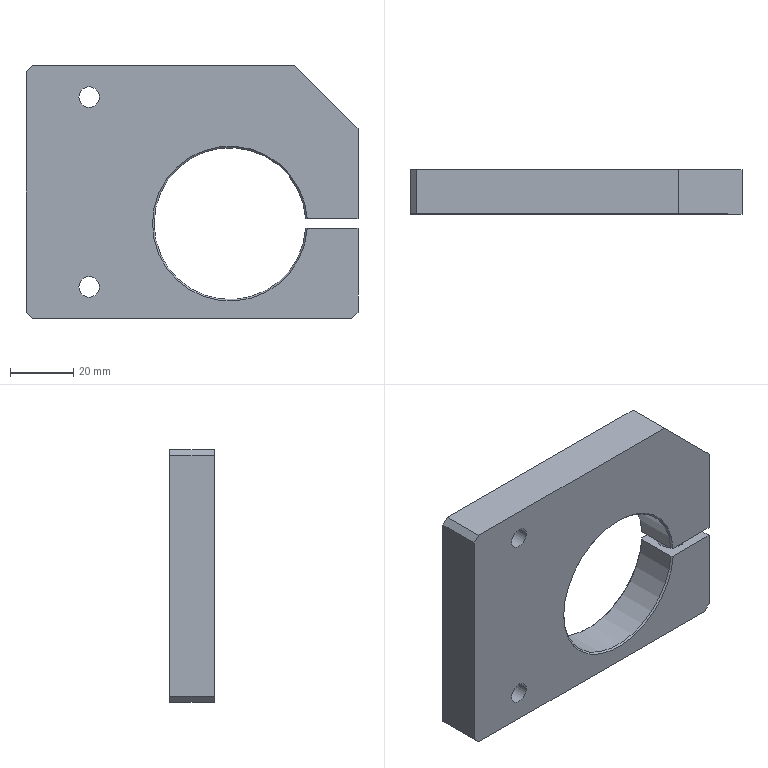Part | NX | 1 solid | 30 faces | box 105 x 14 x 80 mm | volume 85022 mm3 | plane 13 | cylinder 10 | cone 7 | commonest cylinder face diameters 6.5 x4 6.8 x2 9 x2 48 x2
STEP:
#1=CARTESIAN_POINT('',(-50.5,-7.,-40.));
#2=VERTEX_POINT('',#1);
#3=CARTESIAN_POINT('',(-50.5,7.,-40.));
#4=VERTEX_POINT('',#3);
#5=CARTESIAN_POINT('',(-50.5,-7.,-40.));
#6=DIRECTION('',(0.,1.,0.));
#7=VECTOR('',#6,1000.);
#8=LINE('',#5,#7);
#9=EDGE_CURVE('',#2,#4,#8,.T.);
#10=ORIENTED_EDGE('',*,*,#9,.T.);
#11=CARTESIAN_POINT('',(50.5,7.,-40.));
#12=VERTEX_POINT('',#11);
#13=CARTESIAN_POINT('',(-50.5,7.,-40.));
#14=DIRECTION('',(1.,0.,0.));
#15=VECTOR('',#14,1000.);
#16=LINE('',#13,#15);
#17=EDGE_CURVE('',#4,#12,#16,.T.);
#18=ORIENTED_EDGE('',*,*,#17,.T.);
#19=CARTESIAN_POINT('',(50.5,-7.,-40.));
#20=VERTEX_POINT('',#19);
#21=CARTESIAN_POINT('',(50.5,7.,-40.));
#22=DIRECTION('',(0.,-1.,0.));
#23=VECTOR('',#22,1000.);
#24=LINE('',#21,#23);
#25=EDGE_CURVE('',#12,#20,#24,.T.);
#26=ORIENTED_EDGE('',*,*,#25,.T.);
#27=CARTESIAN_POINT('',(50.5,-7.,-40.));
#28=DIRECTION('',(-1.,0.,0.));
#29=VECTOR('',#28,1000.);
#30=LINE('',#27,#29);
#31=EDGE_CURVE('',#20,#2,#30,.T.);
#32=ORIENTED_EDGE('',*,*,#31,.T.);
#33=EDGE_LOOP('',(#10,#18,#26,#32));
#34=FACE_BOUND('',#33,.T.);
#35=CARTESIAN_POINT('',(47.,0.,-40.));
#36=VERTEX_POINT('',#35);
#37=CARTESIAN_POINT('',(38.,0.,-40.));
#38=VERTEX_POINT('',#37);
#39=CARTESIAN_POINT('',(42.5,0.,-40.));
#40=DIRECTION('',(0.,0.,-1.));
#41=DIRECTION('',(1.,0.,0.));
#42=AXIS2_PLACEMENT_3D('',#39,#40,#41);
#43=CIRCLE('',#42,4.5);
#44=EDGE_CURVE('',#36,#38,#43,.T.);
#45=ORIENTED_EDGE('',*,*,#44,.F.);
#46=CARTESIAN_POINT('',(42.5,0.,-40.));
#47=DIRECTION('',(0.,0.,-1.));
#48=DIRECTION('',(1.,0.,0.));
#49=AXIS2_PLACEMENT_3D('',#46,#47,#48);
#50=CIRCLE('',#49,4.5);
#51=EDGE_CURVE('',#38,#36,#50,.T.);
#52=ORIENTED_EDGE('',*,*,#51,.F.);
#53=EDGE_LOOP('',(#45,#52));
#54=FACE_BOUND('',#53,.T.);
#55=CARTESIAN_POINT('',(0.,0.,-40.));
#56=DIRECTION('',(0.,0.,1.));
#57=DIRECTION('',(1.,0.,0.));
#58=AXIS2_PLACEMENT_3D('',#55,#56,#57);
#59=PLANE('',#58);
#60=ADVANCED_FACE('',(#34,#54),#59,.F.);
#61=ORIENTED_EDGE('',*,*,#9,.F.);
#62=CARTESIAN_POINT('',(-52.5,-7.,-38.));
#63=VERTEX_POINT('',#62);
#64=CARTESIAN_POINT('',(-50.5,-7.,-40.));
#65=DIRECTION('',(-0.7071,0.,0.7071));
#66=VECTOR('',#65,1000.);
#67=LINE('',#64,#66);
#68=EDGE_CURVE('',#2,#63,#67,.T.);
#69=ORIENTED_EDGE('',*,*,#68,.T.);
#70=CARTESIAN_POINT('',(-52.5,7.,-38.));
#71=VERTEX_POINT('',#70);
#72=CARTESIAN_POINT('',(-52.5,-7.,-38.));
#73=DIRECTION('',(0.,1.,0.));
#74=VECTOR('',#73,1000.);
#75=LINE('',#72,#74);
#76=EDGE_CURVE('',#63,#71,#75,.T.);
#77=ORIENTED_EDGE('',*,*,#76,.T.);
#78=CARTESIAN_POINT('',(-52.5,7.,-38.));
#79=DIRECTION('',(0.7071,0.,-0.7071));
#80=VECTOR('',#79,1000.);
#81=LINE('',#78,#80);
#82=EDGE_CURVE('',#71,#4,#81,.T.);
#83=ORIENTED_EDGE('',*,*,#82,.T.);
#84=EDGE_LOOP('',(#61,#69,#77,#83));
#85=FACE_BOUND('',#84,.T.);
#86=CARTESIAN_POINT('',(-50.5,7.,-40.));
#87=DIRECTION('',(-0.7071,0.,-0.7071));
#88=DIRECTION('',(-0.7071,0.,0.7071));
#89=AXIS2_PLACEMENT_3D('',#86,#87,#88);
#90=PLANE('',#89);
#91=ADVANCED_FACE('',(#85),#90,.T.);
#92=CARTESIAN_POINT('',(36.454,7.,-11.5));
#93=VERTEX_POINT('',#92);
#94=CARTESIAN_POINT('',(52.5,7.,-11.5));
#95=VERTEX_POINT('',#94);
#96=CARTESIAN_POINT('',(36.454,7.,-11.5));
#97=DIRECTION('',(1.,0.,0.));
#98=VECTOR('',#97,1000.);
#99=LINE('',#96,#98);
#100=EDGE_CURVE('',#93,#95,#99,.T.);
#101=ORIENTED_EDGE('',*,*,#100,.T.);
#102=CARTESIAN_POINT('',(52.5,7.,-38.));
#103=VERTEX_POINT('',#102);
#104=CARTESIAN_POINT('',(52.5,7.,-11.5));
#105=DIRECTION('',(0.,0.,-1.));
#106=VECTOR('',#105,1000.);
#107=LINE('',#104,#106);
#108=EDGE_CURVE('',#95,#103,#107,.T.);
#109=ORIENTED_EDGE('',*,*,#108,.T.);
#110=CARTESIAN_POINT('',(50.5,7.,-40.));
#111=DIRECTION('',(0.7071,0.,0.7071));
#112=VECTOR('',#111,1000.);
#113=LINE('',#110,#112);
#114=EDGE_CURVE('',#12,#103,#113,.T.);
#115=ORIENTED_EDGE('',*,*,#114,.F.);
#116=ORIENTED_EDGE('',*,*,#17,.F.);
#117=ORIENTED_EDGE('',*,*,#82,.F.);
#118=CARTESIAN_POINT('',(-52.5,7.,38.));
#119=VERTEX_POINT('',#118);
#120=CARTESIAN_POINT('',(-52.5,7.,38.));
#121=DIRECTION('',(0.,0.,-1.));
#122=VECTOR('',#121,1000.);
#123=LINE('',#120,#122);
#124=EDGE_CURVE('',#119,#71,#123,.T.);
#125=ORIENTED_EDGE('',*,*,#124,.F.);
#126=CARTESIAN_POINT('',(-50.5,7.,40.));
#127=VERTEX_POINT('',#126);
#128=CARTESIAN_POINT('',(-50.5,7.,40.));
#129=DIRECTION('',(-0.7071,0.,-0.7071));
#130=VECTOR('',#129,1000.);
#131=LINE('',#128,#130);
#132=EDGE_CURVE('',#127,#119,#131,.T.);
#133=ORIENTED_EDGE('',*,*,#132,.F.);
#134=CARTESIAN_POINT('',(32.5,7.,40.));
#135=VERTEX_POINT('',#134);
#136=CARTESIAN_POINT('',(-50.5,7.,40.));
#137=DIRECTION('',(1.,0.,0.));
#138=VECTOR('',#137,1000.);
#139=LINE('',#136,#138);
#140=EDGE_CURVE('',#127,#135,#139,.T.);
#141=ORIENTED_EDGE('',*,*,#140,.T.);
#142=CARTESIAN_POINT('',(52.5,7.,20.));
#143=VERTEX_POINT('',#142);
#144=CARTESIAN_POINT('',(52.5,7.,20.));
#145=DIRECTION('',(-0.7071,0.,0.7071));
#146=VECTOR('',#145,1000.);
#147=LINE('',#144,#146);
#148=EDGE_CURVE('',#143,#135,#147,.T.);
#149=ORIENTED_EDGE('',*,*,#148,.F.);
#150=CARTESIAN_POINT('',(52.5,7.,-8.5));
#151=VERTEX_POINT('',#150);
#152=CARTESIAN_POINT('',(52.5,7.,20.));
#153=DIRECTION('',(0.,0.,-1.));
#154=VECTOR('',#153,1000.);
#155=LINE('',#152,#154);
#156=EDGE_CURVE('',#143,#151,#155,.T.);
#157=ORIENTED_EDGE('',*,*,#156,.T.);
#158=CARTESIAN_POINT('',(36.454,7.,-8.5));
#159=VERTEX_POINT('',#158);
#160=CARTESIAN_POINT('',(0.,7.,-8.5));
#161=DIRECTION('',(1.,0.,0.));
#162=VECTOR('',#161,1000.);
#163=LINE('',#160,#162);
#164=EDGE_CURVE('',#159,#151,#163,.T.);
#165=ORIENTED_EDGE('',*,*,#164,.F.);
#166=CARTESIAN_POINT('',(12.,7.,-10.));
#167=DIRECTION('',(0.,1.,0.));
#168=DIRECTION('',(-1.,0.,0.));
#169=AXIS2_PLACEMENT_3D('',#166,#167,#168);
#170=CIRCLE('',#169,24.5);
#171=EDGE_CURVE('',#93,#159,#170,.T.);
#172=ORIENTED_EDGE('',*,*,#171,.F.);
#173=EDGE_LOOP('',(#101,#109,#115,#116,#117,#125,#133,#141,#149,#157,#165,#172));
#174=FACE_BOUND('',#173,.T.);
#175=CARTESIAN_POINT('',(-35.75,7.,30.));
#176=VERTEX_POINT('',#175);
#177=CARTESIAN_POINT('',(-29.25,7.,30.));
#178=VERTEX_POINT('',#177);
#179=CARTESIAN_POINT('',(-32.5,7.,30.));
#180=DIRECTION('',(0.,1.,0.));
#181=DIRECTION('',(1.,0.,0.));
#182=AXIS2_PLACEMENT_3D('',#179,#180,#181);
#183=CIRCLE('',#182,3.25);
#184=EDGE_CURVE('',#176,#178,#183,.T.);
#185=ORIENTED_EDGE('',*,*,#184,.F.);
#186=CARTESIAN_POINT('',(-32.5,7.,30.));
#187=DIRECTION('',(0.,1.,0.));
#188=DIRECTION('',(1.,0.,0.));
#189=AXIS2_PLACEMENT_3D('',#186,#187,#188);
#190=CIRCLE('',#189,3.25);
#191=EDGE_CURVE('',#178,#176,#190,.T.);
#192=ORIENTED_EDGE('',*,*,#191,.F.);
#193=EDGE_LOOP('',(#185,#192));
#194=FACE_BOUND('',#193,.T.);
#195=CARTESIAN_POINT('',(-29.25,7.,-30.));
#196=VERTEX_POINT('',#195);
#197=CARTESIAN_POINT('',(-35.75,7.,-30.));
#198=VERTEX_POINT('',#197);
#199=CARTESIAN_POINT('',(-32.5,7.,-30.));
#200=DIRECTION('',(0.,1.,0.));
#201=DIRECTION('',(1.,0.,0.));
#202=AXIS2_PLACEMENT_3D('',#199,#200,#201);
#203=CIRCLE('',#202,3.25);
#204=EDGE_CURVE('',#196,#198,#203,.T.);
#205=ORIENTED_EDGE('',*,*,#204,.F.);
#206=CARTESIAN_POINT('',(-32.5,7.,-30.));
#207=DIRECTION('',(0.,1.,0.));
#208=DIRECTION('',(1.,0.,0.));
#209=AXIS2_PLACEMENT_3D('',#206,#207,#208);
#210=CIRCLE('',#209,3.25);
#211=EDGE_CURVE('',#198,#196,#210,.T.);
#212=ORIENTED_EDGE('',*,*,#211,.F.);
#213=EDGE_LOOP('',(#205,#212));
#214=FACE_BOUND('',#213,.T.);
#215=CARTESIAN_POINT('',(52.5,7.,-40.));
#216=DIRECTION('',(0.,1.,0.));
#217=DIRECTION('',(1.,0.,0.));
#218=AXIS2_PLACEMENT_3D('',#215,#216,#217);
#219=PLANE('',#218);
#220=ADVANCED_FACE('',(#174,#194,#214),#219,.T.);
#221=CARTESIAN_POINT('',(36.454,-7.,-11.5));
#222=VERTEX_POINT('',#221);
#223=CARTESIAN_POINT('',(52.5,-7.,-11.5));
#224=VERTEX_POINT('',#223);
#225=CARTESIAN_POINT('',(36.454,-7.,-11.5));
#226=DIRECTION('',(1.,0.,0.));
#227=VECTOR('',#226,1000.);
#228=LINE('',#225,#227);
#229=EDGE_CURVE('',#222,#224,#228,.T.);
#230=ORIENTED_EDGE('',*,*,#229,.T.);
#231=CARTESIAN_POINT('',(52.5,7.,-11.5));
#232=DIRECTION('',(0.,-1.,0.));
#233=VECTOR('',#232,1000.);
#234=LINE('',#231,#233);
#235=EDGE_CURVE('',#95,#224,#234,.T.);
#236=ORIENTED_EDGE('',*,*,#235,.F.);
#237=ORIENTED_EDGE('',*,*,#100,.F.);
#238=CARTESIAN_POINT('',(35.953,6.5,-11.5));
#239=VERTEX_POINT('',#238);
#240=CARTESIAN_POINT('',(36.454,7.,-11.5));
#241=CARTESIAN_POINT('',(36.398,6.944,-11.5));
#242=CARTESIAN_POINT('',(36.287,6.833,-11.5));
#243=CARTESIAN_POINT('',(36.12,6.667,-11.5));
#244=CARTESIAN_POINT('',(36.009,6.556,-11.5));
#245=CARTESIAN_POINT('',(35.953,6.5,-11.5));
#246=B_SPLINE_CURVE_WITH_KNOTS('',3,(#240,#241,#242,#243,#244,#245),.UNSPECIFIED.,.F.,.F.,(4,1,1,4),(0.,0.3333,0.6667,1.),.UNSPECIFIED.);
#247=EDGE_CURVE('',#93,#239,#246,.T.);
#248=ORIENTED_EDGE('',*,*,#247,.T.);
#249=CARTESIAN_POINT('',(35.953,-6.5,-11.5));
#250=VERTEX_POINT('',#249);
#251=CARTESIAN_POINT('',(35.953,6.5,-11.5));
#252=DIRECTION('',(0.,-1.,0.));
#253=VECTOR('',#252,1000.);
#254=LINE('',#251,#253);
#255=EDGE_CURVE('',#239,#250,#254,.T.);
#256=ORIENTED_EDGE('',*,*,#255,.T.);
#257=CARTESIAN_POINT('',(35.953,-6.5,-11.5));
#258=CARTESIAN_POINT('',(36.009,-6.556,-11.5));
#259=CARTESIAN_POINT('',(36.12,-6.667,-11.5));
#260=CARTESIAN_POINT('',(36.287,-6.833,-11.5));
#261=CARTESIAN_POINT('',(36.398,-6.944,-11.5));
#262=CARTESIAN_POINT('',(36.454,-7.,-11.5));
#263=B_SPLINE_CURVE_WITH_KNOTS('',3,(#257,#258,#259,#260,#261,#262),.UNSPECIFIED.,.F.,.F.,(4,1,1,4),(0.,0.3333,0.6667,1.),.UNSPECIFIED.);
#264=EDGE_CURVE('',#250,#222,#263,.T.);
#265=ORIENTED_EDGE('',*,*,#264,.T.);
#266=EDGE_LOOP('',(#230,#236,#237,#248,#256,#265));
#267=FACE_BOUND('',#266,.T.);
#268=CARTESIAN_POINT('',(47.,0.,-11.5));
#269=VERTEX_POINT('',#268);
#270=CARTESIAN_POINT('',(38.,0.,-11.5));
#271=VERTEX_POINT('',#270);
#272=CARTESIAN_POINT('',(42.5,0.,-11.5));
#273=DIRECTION('',(0.,0.,1.));
#274=DIRECTION('',(-1.,0.,0.));
#275=AXIS2_PLACEMENT_3D('',#272,#273,#274);
#276=CIRCLE('',#275,4.5);
#277=EDGE_CURVE('',#269,#271,#276,.T.);
#278=ORIENTED_EDGE('',*,*,#277,.F.);
#279=CARTESIAN_POINT('',(42.5,0.,-11.5));
#280=DIRECTION('',(0.,0.,1.));
#281=DIRECTION('',(-1.,0.,0.));
#282=AXIS2_PLACEMENT_3D('',#279,#280,#281);
#283=CIRCLE('',#282,4.5);
#284=EDGE_CURVE('',#271,#269,#283,.T.);
#285=ORIENTED_EDGE('',*,*,#284,.F.);
#286=EDGE_LOOP('',(#278,#285));
#287=FACE_BOUND('',#286,.T.);
#288=CARTESIAN_POINT('',(52.5,7.,-11.5));
#289=DIRECTION('',(0.,0.,-1.));
#290=DIRECTION('',(0.,-1.,0.));
#291=AXIS2_PLACEMENT_3D('',#288,#289,#290);
#292=PLANE('',#291);
#293=ADVANCED_FACE('',(#267,#287),#292,.F.);
#294=ORIENTED_EDGE('',*,*,#229,.F.);
#295=CARTESIAN_POINT('',(-12.5,-7.,-10.));
#296=VERTEX_POINT('',#295);
#297=CARTESIAN_POINT('',(12.,-7.,-10.));
#298=DIRECTION('',(0.,-1.,0.));
#299=DIRECTION('',(-1.,0.,0.));
#300=AXIS2_PLACEMENT_3D('',#297,#298,#299);
#301=CIRCLE('',#300,24.5);
#302=EDGE_CURVE('',#296,#222,#301,.T.);
#303=ORIENTED_EDGE('',*,*,#302,.F.);
#304=CARTESIAN_POINT('',(36.454,-7.,-8.5));
#305=VERTEX_POINT('',#304);
#306=CARTESIAN_POINT('',(12.,-7.,-10.));
#307=DIRECTION('',(0.,-1.,0.));
#308=DIRECTION('',(-1.,0.,0.));
#309=AXIS2_PLACEMENT_3D('',#306,#307,#308);
#310=CIRCLE('',#309,24.5);
#311=EDGE_CURVE('',#305,#296,#310,.T.);
#312=ORIENTED_EDGE('',*,*,#311,.F.);
#313=CARTESIAN_POINT('',(52.5,-7.,-8.5));
#314=VERTEX_POINT('',#313);
#315=CARTESIAN_POINT('',(0.,-7.,-8.5));
#316=DIRECTION('',(-1.,0.,0.));
#317=VECTOR('',#316,1000.);
#318=LINE('',#315,#317);
#319=EDGE_CURVE('',#314,#305,#318,.T.);
#320=ORIENTED_EDGE('',*,*,#319,.F.);
#321=CARTESIAN_POINT('',(52.5,-7.,20.));
#322=VERTEX_POINT('',#321);
#323=CARTESIAN_POINT('',(52.5,-7.,20.));
#324=DIRECTION('',(0.,0.,-1.));
#325=VECTOR('',#324,1000.);
#326=LINE('',#323,#325);
#327=EDGE_CURVE('',#322,#314,#326,.T.);
#328=ORIENTED_EDGE('',*,*,#327,.F.);
#329=CARTESIAN_POINT('',(32.5,-7.,40.));
#330=VERTEX_POINT('',#329);
#331=CARTESIAN_POINT('',(32.5,-7.,40.));
#332=DIRECTION('',(0.7071,0.,-0.7071));
#333=VECTOR('',#332,1000.);
#334=LINE('',#331,#333);
#335=EDGE_CURVE('',#330,#322,#334,.T.);
#336=ORIENTED_EDGE('',*,*,#335,.F.);
#337=CARTESIAN_POINT('',(-50.5,-7.,40.));
#338=VERTEX_POINT('',#337);
#339=CARTESIAN_POINT('',(32.5,-7.,40.));
#340=DIRECTION('',(-1.,0.,0.));
#341=VECTOR('',#340,1000.);
#342=LINE('',#339,#341);
#343=EDGE_CURVE('',#330,#338,#342,.T.);
#344=ORIENTED_EDGE('',*,*,#343,.T.);
#345=CARTESIAN_POINT('',(-52.5,-7.,38.));
#346=VERTEX_POINT('',#345);
#347=CARTESIAN_POINT('',(-52.5,-7.,38.));
#348=DIRECTION('',(0.7071,0.,0.7071));
#349=VECTOR('',#348,1000.);
#350=LINE('',#347,#349);
#351=EDGE_CURVE('',#346,#338,#350,.T.);
#352=ORIENTED_EDGE('',*,*,#351,.F.);
#353=CARTESIAN_POINT('',(-52.5,-7.,38.));
#354=DIRECTION('',(0.,0.,-1.));
#355=VECTOR('',#354,1000.);
#356=LINE('',#353,#355);
#357=EDGE_CURVE('',#346,#63,#356,.T.);
#358=ORIENTED_EDGE('',*,*,#357,.T.);
#359=ORIENTED_EDGE('',*,*,#68,.F.);
#360=ORIENTED_EDGE('',*,*,#31,.F.);
#361=CARTESIAN_POINT('',(52.5,-7.,-38.));
#362=VERTEX_POINT('',#361);
#363=CARTESIAN_POINT('',(52.5,-7.,-38.));
#364=DIRECTION('',(-0.7071,0.,-0.7071));
#365=VECTOR('',#364,1000.);
#366=LINE('',#363,#365);
#367=EDGE_CURVE('',#362,#20,#366,.T.);
#368=ORIENTED_EDGE('',*,*,#367,.F.);
#369=CARTESIAN_POINT('',(52.5,-7.,-11.5));
#370=DIRECTION('',(0.,0.,-1.));
#371=VECTOR('',#370,1000.);
#372=LINE('',#369,#371);
#373=EDGE_CURVE('',#224,#362,#372,.T.);
#374=ORIENTED_EDGE('',*,*,#373,.F.);
#375=EDGE_LOOP('',(#294,#303,#312,#320,#328,#336,#344,#352,#358,#359,#360,#368,#374));
#376=FACE_BOUND('',#375,.T.);
#377=CARTESIAN_POINT('',(-35.75,-7.,30.));
#378=VERTEX_POINT('',#377);
#379=CARTESIAN_POINT('',(-29.25,-7.,30.));
#380=VERTEX_POINT('',#379);
#381=CARTESIAN_POINT('',(-32.5,-7.,30.));
#382=DIRECTION('',(0.,-1.,0.));
#383=DIRECTION('',(-1.,0.,0.));
#384=AXIS2_PLACEMENT_3D('',#381,#382,#383);
#385=CIRCLE('',#384,3.25);
#386=EDGE_CURVE('',#378,#380,#385,.T.);
#387=ORIENTED_EDGE('',*,*,#386,.F.);
#388=CARTESIAN_POINT('',(-32.5,-7.,30.));
#389=DIRECTION('',(0.,-1.,0.));
#390=DIRECTION('',(-1.,0.,0.));
#391=AXIS2_PLACEMENT_3D('',#388,#389,#390);
#392=CIRCLE('',#391,3.25);
#393=EDGE_CURVE('',#380,#378,#392,.T.);
#394=ORIENTED_EDGE('',*,*,#393,.F.);
#395=EDGE_LOOP('',(#387,#394));
#396=FACE_BOUND('',#395,.T.);
#397=CARTESIAN_POINT('',(-29.25,-7.,-30.));
#398=VERTEX_POINT('',#397);
#399=CARTESIAN_POINT('',(-35.75,-7.,-30.));
#400=VERTEX_POINT('',#399);
#401=CARTESIAN_POINT('',(-32.5,-7.,-30.));
#402=DIRECTION('',(0.,-1.,0.));
#403=DIRECTION('',(-1.,0.,0.));
#404=AXIS2_PLACEMENT_3D('',#401,#402,#403);
#405=CIRCLE('',#404,3.25);
#406=EDGE_CURVE('',#398,#400,#405,.T.);
#407=ORIENTED_EDGE('',*,*,#406,.F.);
#408=CARTESIAN_POINT('',(-32.5,-7.,-30.));
#409=DIRECTION('',(0.,-1.,0.));
#410=DIRECTION('',(-1.,0.,0.));
#411=AXIS2_PLACEMENT_3D('',#408,#409,#410);
#412=CIRCLE('',#411,3.25);
#413=EDGE_CURVE('',#400,#398,#412,.T.);
#414=ORIENTED_EDGE('',*,*,#413,.F.);
#415=EDGE_LOOP('',(#407,#414));
#416=FACE_BOUND('',#415,.T.);
#417=CARTESIAN_POINT('',(-52.5,-7.,-40.));
#418=DIRECTION('',(0.,-1.,0.));
#419=DIRECTION('',(0.,0.,-1.));
#420=AXIS2_PLACEMENT_3D('',#417,#418,#419);
#421=PLANE('',#420);
#422=ADVANCED_FACE('',(#376,#396,#416),#421,.T.);
#423=ORIENTED_EDGE('',*,*,#235,.T.);
#424=ORIENTED_EDGE('',*,*,#373,.T.);
#425=CARTESIAN_POINT('',(52.5,7.,-38.));
#426=DIRECTION('',(0.,-1.,0.));
#427=VECTOR('',#426,1000.);
#428=LINE('',#425,#427);
#429=EDGE_CURVE('',#103,#362,#428,.T.);
#430=ORIENTED_EDGE('',*,*,#429,.F.);
#431=ORIENTED_EDGE('',*,*,#108,.F.);
#432=EDGE_LOOP('',(#423,#424,#430,#431));
#433=FACE_BOUND('',#432,.T.);
#434=CARTESIAN_POINT('',(52.5,-7.,-40.));
#435=DIRECTION('',(1.,0.,0.));
#436=DIRECTION('',(0.,1.,0.));
#437=AXIS2_PLACEMENT_3D('',#434,#435,#436);
#438=PLANE('',#437);
#439=ADVANCED_FACE('',(#433),#438,.T.);
#440=ORIENTED_EDGE('',*,*,#25,.F.);
#441=ORIENTED_EDGE('',*,*,#114,.T.);
#442=ORIENTED_EDGE('',*,*,#429,.T.);
#443=ORIENTED_EDGE('',*,*,#367,.T.);
#444=EDGE_LOOP('',(#440,#441,#442,#443));
#445=FACE_BOUND('',#444,.T.);
#446=CARTESIAN_POINT('',(50.5,-7.,-40.));
#447=DIRECTION('',(0.7071,0.,-0.7071));
#448=DIRECTION('',(0.,-1.,0.));
#449=AXIS2_PLACEMENT_3D('',#446,#447,#448);
#450=PLANE('',#449);
#451=ADVANCED_FACE('',(#445),#450,.T.);
#452=ORIENTED_EDGE('',*,*,#76,.F.);
#453=ORIENTED_EDGE('',*,*,#357,.F.);
#454=CARTESIAN_POINT('',(-52.5,-7.,38.));
#455=DIRECTION('',(0.,1.,0.));
#456=VECTOR('',#455,1000.);
#457=LINE('',#454,#456);
#458=EDGE_CURVE('',#346,#119,#457,.T.);
#459=ORIENTED_EDGE('',*,*,#458,.T.);
#460=ORIENTED_EDGE('',*,*,#124,.T.);
#461=EDGE_LOOP('',(#452,#453,#459,#460));
#462=FACE_BOUND('',#461,.T.);
#463=CARTESIAN_POINT('',(-52.5,7.,-40.));
#464=DIRECTION('',(-1.,0.,0.));
#465=DIRECTION('',(0.,0.,1.));
#466=AXIS2_PLACEMENT_3D('',#463,#464,#465);
#467=PLANE('',#466);
#468=ADVANCED_FACE('',(#462),#467,.T.);
#469=CARTESIAN_POINT('',(-50.5,-7.,40.));
#470=DIRECTION('',(0.,1.,0.));
#471=VECTOR('',#470,1000.);
#472=LINE('',#469,#471);
#473=EDGE_CURVE('',#338,#127,#472,.T.);
#474=ORIENTED_EDGE('',*,*,#473,.T.);
#475=ORIENTED_EDGE('',*,*,#132,.T.);
#476=ORIENTED_EDGE('',*,*,#458,.F.);
#477=ORIENTED_EDGE('',*,*,#351,.T.);
#478=EDGE_LOOP('',(#474,#475,#476,#477));
#479=FACE_BOUND('',#478,.T.);
#480=CARTESIAN_POINT('',(-50.5,7.,40.));
#481=DIRECTION('',(0.7071,0.,-0.7071));
#482=DIRECTION('',(0.,-1.,0.));
#483=AXIS2_PLACEMENT_3D('',#480,#481,#482);
#484=PLANE('',#483);
#485=ADVANCED_FACE('',(#479),#484,.F.);
#486=ORIENTED_EDGE('',*,*,#473,.F.);
#487=ORIENTED_EDGE('',*,*,#343,.F.);
#488=CARTESIAN_POINT('',(32.5,7.,40.));
#489=DIRECTION('',(0.,-1.,0.));
#490=VECTOR('',#489,1000.);
#491=LINE('',#488,#490);
#492=EDGE_CURVE('',#135,#330,#491,.T.);
#493=ORIENTED_EDGE('',*,*,#492,.F.);
#494=ORIENTED_EDGE('',*,*,#140,.F.);
#495=EDGE_LOOP('',(#486,#487,#493,#494));
#496=FACE_BOUND('',#495,.T.);
#497=CARTESIAN_POINT('',(0.,0.,40.));
#498=DIRECTION('',(0.,0.,1.));
#499=DIRECTION('',(1.,0.,0.));
#500=AXIS2_PLACEMENT_3D('',#497,#498,#499);
#501=PLANE('',#500);
#502=ADVANCED_FACE('',(#496),#501,.T.);
#503=ORIENTED_EDGE('',*,*,#492,.T.);
#504=ORIENTED_EDGE('',*,*,#335,.T.);
#505=CARTESIAN_POINT('',(52.5,7.,20.));
#506=DIRECTION('',(0.,-1.,0.));
#507=VECTOR('',#506,1000.);
#508=LINE('',#505,#507);
#509=EDGE_CURVE('',#143,#322,#508,.T.);
#510=ORIENTED_EDGE('',*,*,#509,.F.);
#511=ORIENTED_EDGE('',*,*,#148,.T.);
#512=EDGE_LOOP('',(#503,#504,#510,#511));
#513=FACE_BOUND('',#512,.T.);
#514=CARTESIAN_POINT('',(32.5,-7.,40.));
#515=DIRECTION('',(-0.7071,0.,-0.7071));
#516=DIRECTION('',(-0.7071,0.,0.7071));
#517=AXIS2_PLACEMENT_3D('',#514,#515,#516);
#518=PLANE('',#517);
#519=ADVANCED_FACE('',(#513),#518,.F.);
#520=CARTESIAN_POINT('',(52.5,0.,-8.5));
#521=DIRECTION('',(0.,-1.,0.));
#522=VECTOR('',#521,1000.);
#523=LINE('',#520,#522);
#524=EDGE_CURVE('',#151,#314,#523,.T.);
#525=ORIENTED_EDGE('',*,*,#524,.F.);
#526=ORIENTED_EDGE('',*,*,#156,.F.);
#527=ORIENTED_EDGE('',*,*,#509,.T.);
#528=ORIENTED_EDGE('',*,*,#327,.T.);
#529=EDGE_LOOP('',(#525,#526,#527,#528));
#530=FACE_BOUND('',#529,.T.);
#531=CARTESIAN_POINT('',(52.5,-7.,-40.));
#532=DIRECTION('',(1.,0.,0.));
#533=DIRECTION('',(0.,1.,0.));
#534=AXIS2_PLACEMENT_3D('',#531,#532,#533);
#535=PLANE('',#534);
#536=ADVANCED_FACE('',(#530),#535,.T.);
#537=ORIENTED_EDGE('',*,*,#319,.T.);
#538=CARTESIAN_POINT('',(35.953,-6.5,-8.5));
#539=VERTEX_POINT('',#538);
#540=CARTESIAN_POINT('',(35.953,-6.5,-8.5));
#541=CARTESIAN_POINT('',(35.995,-6.542,-8.5));
#542=CARTESIAN_POINT('',(36.037,-6.583,-8.5));
#543=CARTESIAN_POINT('',(36.078,-6.625,-8.5));
#544=CARTESIAN_POINT('',(36.12,-6.667,-8.5));
#545=CARTESIAN_POINT('',(36.162,-6.708,-8.5));
#546=CARTESIAN_POINT('',(36.204,-6.75,-8.5));
#547=CARTESIAN_POINT('',(36.245,-6.792,-8.5));
#548=CARTESIAN_POINT('',(36.287,-6.833,-8.5));
#549=CARTESIAN_POINT('',(36.329,-6.875,-8.5));
#550=CARTESIAN_POINT('',(36.371,-6.917,-8.5));
#551=CARTESIAN_POINT('',(36.412,-6.958,-8.5));
#552=CARTESIAN_POINT('',(36.454,-7.,-8.5));
#553=B_SPLINE_CURVE_WITH_KNOTS('',3,(#540,#541,#542,#543,#544,#545,#546,#547,#548,#549,#550,#551,#552),.UNSPECIFIED.,.F.,.F.,(4,3,3,3,4),(0.,0.1769,0.3539,0.5308,0.7078),.UNSPECIFIED.);
#554=EDGE_CURVE('',#539,#305,#553,.T.);
#555=ORIENTED_EDGE('',*,*,#554,.F.);
#556=CARTESIAN_POINT('',(35.953,6.5,-8.5));
#557=VERTEX_POINT('',#556);
#558=CARTESIAN_POINT('',(35.953,-7.,-8.5));
#559=DIRECTION('',(0.,1.,0.));
#560=VECTOR('',#559,1000.);
#561=LINE('',#558,#560);
#562=EDGE_CURVE('',#539,#557,#561,.T.);
#563=ORIENTED_EDGE('',*,*,#562,.T.);
#564=CARTESIAN_POINT('',(36.454,7.,-8.5));
#565=CARTESIAN_POINT('',(36.412,6.958,-8.5));
#566=CARTESIAN_POINT('',(36.371,6.917,-8.5));
#567=CARTESIAN_POINT('',(36.329,6.875,-8.5));
#568=CARTESIAN_POINT('',(36.287,6.833,-8.5));
#569=CARTESIAN_POINT('',(36.245,6.792,-8.5));
#570=CARTESIAN_POINT('',(36.204,6.75,-8.5));
#571=CARTESIAN_POINT('',(36.162,6.708,-8.5));
#572=CARTESIAN_POINT('',(36.12,6.667,-8.5));
#573=CARTESIAN_POINT('',(36.078,6.625,-8.5));
#574=CARTESIAN_POINT('',(36.057,6.604,-8.5));
#575=CARTESIAN_POINT('',(36.037,6.583,-8.5));
#576=CARTESIAN_POINT('',(36.016,6.562,-8.5));
#577=CARTESIAN_POINT('',(35.995,6.542,-8.5));
#578=CARTESIAN_POINT('',(35.974,6.521,-8.5));
#579=CARTESIAN_POINT('',(35.953,6.5,-8.5));
#580=B_SPLINE_CURVE_WITH_KNOTS('',3,(#564,#565,#566,#567,#568,#569,#570,#571,#572,#573,#574,#575,#576,#577,#578,#579),.UNSPECIFIED.,.F.,.F.,(4,3,3,3,3,4),(0.,0.1769,0.3539,0.5308,0.6193,0.7078),.UNSPECIFIED.);
#581=EDGE_CURVE('',#159,#557,#580,.T.);
#582=ORIENTED_EDGE('',*,*,#581,.F.);
#583=ORIENTED_EDGE('',*,*,#164,.T.);
#584=ORIENTED_EDGE('',*,*,#524,.T.);
#585=EDGE_LOOP('',(#537,#555,#563,#582,#583,#584));
#586=FACE_BOUND('',#585,.T.);
#587=CARTESIAN_POINT('',(47.062,0.,-8.5));
#588=VERTEX_POINT('',#587);
#589=CARTESIAN_POINT('',(37.938,0.,-8.5));
#590=VERTEX_POINT('',#589);
#591=CARTESIAN_POINT('',(42.5,0.,-8.5));
#592=DIRECTION('',(0.,0.,-1.));
#593=DIRECTION('',(-1.,0.,0.));
#594=AXIS2_PLACEMENT_3D('',#591,#592,#593);
#595=CIRCLE('',#594,4.562);
#596=EDGE_CURVE('',#588,#590,#595,.T.);
#597=ORIENTED_EDGE('',*,*,#596,.F.);
#598=CARTESIAN_POINT('',(42.5,0.,-8.5));
#599=DIRECTION('',(0.,0.,-1.));
#600=DIRECTION('',(-1.,0.,0.));
#601=AXIS2_PLACEMENT_3D('',#598,#599,#600);
#602=CIRCLE('',#601,4.562);
#603=EDGE_CURVE('',#590,#588,#602,.T.);
#604=ORIENTED_EDGE('',*,*,#603,.F.);
#605=EDGE_LOOP('',(#597,#604));
#606=FACE_BOUND('',#605,.T.);
#607=CARTESIAN_POINT('',(17.5,7.,-8.5));
#608=DIRECTION('',(0.,0.,1.));
#609=DIRECTION('',(1.,0.,0.));
#610=AXIS2_PLACEMENT_3D('',#607,#608,#609);
#611=PLANE('',#610);
#612=ADVANCED_FACE('',(#586,#606),#611,.F.);
#613=CARTESIAN_POINT('',(-12.,6.5,-10.));
#614=VERTEX_POINT('',#613);
#615=CARTESIAN_POINT('',(12.,6.5,-10.));
#616=DIRECTION('',(0.,1.,0.));
#617=DIRECTION('',(-1.,0.,0.));
#618=AXIS2_PLACEMENT_3D('',#615,#616,#617);
#619=CIRCLE('',#618,24.);
#620=EDGE_CURVE('',#239,#614,#619,.T.);
#621=ORIENTED_EDGE('',*,*,#620,.F.);
#622=ORIENTED_EDGE('',*,*,#247,.F.);
#623=ORIENTED_EDGE('',*,*,#171,.T.);
#624=ORIENTED_EDGE('',*,*,#581,.T.);
#625=CARTESIAN_POINT('',(12.,6.5,-10.));
#626=DIRECTION('',(0.,1.,0.));
#627=DIRECTION('',(-1.,0.,0.));
#628=AXIS2_PLACEMENT_3D('',#625,#626,#627);
#629=CIRCLE('',#628,24.);
#630=EDGE_CURVE('',#614,#557,#629,.T.);
#631=ORIENTED_EDGE('',*,*,#630,.F.);
#632=EDGE_LOOP('',(#621,#622,#623,#624,#631));
#633=FACE_BOUND('',#632,.T.);
#634=CARTESIAN_POINT('',(12.,6.75,-10.));
#635=DIRECTION('',(0.,1.,0.));
#636=DIRECTION('',(1.,0.,0.));
#637=AXIS2_PLACEMENT_3D('',#634,#635,#636);
#638=CONICAL_SURFACE('',#637,24.25,0.7854);
#639=ADVANCED_FACE('',(#633),#638,.F.);
#640=CARTESIAN_POINT('',(-12.,-6.5,-10.));
#641=VERTEX_POINT('',#640);
#642=CARTESIAN_POINT('',(-12.,-7.,-10.));
#643=DIRECTION('',(0.,1.,0.));
#644=VECTOR('',#643,1000.);
#645=LINE('',#642,#644);
#646=EDGE_CURVE('',#641,#614,#645,.T.);
#647=ORIENTED_EDGE('',*,*,#646,.F.);
#648=CARTESIAN_POINT('',(12.,-6.5,-10.));
#649=DIRECTION('',(0.,-1.,0.));
#650=DIRECTION('',(0.998,0.,0.0625));
#651=AXIS2_PLACEMENT_3D('',#648,#649,#650);
#652=CIRCLE('',#651,24.);
#653=EDGE_CURVE('',#641,#250,#652,.T.);
#654=ORIENTED_EDGE('',*,*,#653,.T.);
#655=ORIENTED_EDGE('',*,*,#255,.F.);
#656=ORIENTED_EDGE('',*,*,#620,.T.);
#657=EDGE_LOOP('',(#647,#654,#655,#656));
#658=FACE_BOUND('',#657,.T.);
#659=CARTESIAN_POINT('',(12.,-7.,-10.));
#660=DIRECTION('',(0.,1.,0.));
#661=DIRECTION('',(-1.,0.,0.));
#662=AXIS2_PLACEMENT_3D('',#659,#660,#661);
#663=CYLINDRICAL_SURFACE('',#662,24.);
#664=ADVANCED_FACE('',(#658),#663,.F.);
#665=CARTESIAN_POINT('',(-12.25,-6.75,-10.));
#666=DIRECTION('',(-0.7071,-0.7071,0.));
#667=VECTOR('',#666,1000.);
#668=LINE('',#665,#667);
#669=EDGE_CURVE('',#641,#296,#668,.T.);
#670=ORIENTED_EDGE('',*,*,#669,.F.);
#671=CARTESIAN_POINT('',(12.,-6.5,-10.));
#672=DIRECTION('',(0.,-1.,0.));
#673=DIRECTION('',(0.998,0.,0.0625));
#674=AXIS2_PLACEMENT_3D('',#671,#672,#673);
#675=CIRCLE('',#674,24.);
#676=EDGE_CURVE('',#539,#641,#675,.T.);
#677=ORIENTED_EDGE('',*,*,#676,.F.);
#678=ORIENTED_EDGE('',*,*,#554,.T.);
#679=ORIENTED_EDGE('',*,*,#311,.T.);
#680=EDGE_LOOP('',(#670,#677,#678,#679));
#681=FACE_BOUND('',#680,.T.);
#682=CARTESIAN_POINT('',(12.,-6.75,-10.));
#683=DIRECTION('',(0.,-1.,0.));
#684=DIRECTION('',(-1.,0.,0.));
#685=AXIS2_PLACEMENT_3D('',#682,#683,#684);
#686=CONICAL_SURFACE('',#685,24.25,0.7854);
#687=ADVANCED_FACE('',(#681),#686,.F.);
#688=ORIENTED_EDGE('',*,*,#406,.T.);
#689=CARTESIAN_POINT('',(-35.75,7.,-30.));
#690=DIRECTION('',(0.,-1.,0.));
#691=VECTOR('',#690,1000.);
#692=LINE('',#689,#691);
#693=EDGE_CURVE('',#400,#198,#692,.F.);
#694=ORIENTED_EDGE('',*,*,#693,.T.);
#695=ORIENTED_EDGE('',*,*,#211,.T.);
#696=CARTESIAN_POINT('',(-29.25,7.,-30.));
#697=DIRECTION('',(0.,-1.,0.));
#698=VECTOR('',#697,1000.);
#699=LINE('',#696,#698);
#700=EDGE_CURVE('',#398,#196,#699,.F.);
#701=ORIENTED_EDGE('',*,*,#700,.F.);
#702=EDGE_LOOP('',(#688,#694,#695,#701));
#703=FACE_BOUND('',#702,.T.);
#704=CARTESIAN_POINT('',(-32.5,7.,-30.));
#705=DIRECTION('',(0.,-1.,0.));
#706=DIRECTION('',(1.,0.,0.));
#707=AXIS2_PLACEMENT_3D('',#704,#705,#706);
#708=CYLINDRICAL_SURFACE('',#707,3.25);
#709=ADVANCED_FACE('',(#703),#708,.F.);
#710=ORIENTED_EDGE('',*,*,#44,.T.);
#711=CARTESIAN_POINT('',(38.,0.,-40.));
#712=DIRECTION('',(0.,0.,1.));
#713=VECTOR('',#712,1000.);
#714=LINE('',#711,#713);
#715=EDGE_CURVE('',#271,#38,#714,.F.);
#716=ORIENTED_EDGE('',*,*,#715,.F.);
#717=ORIENTED_EDGE('',*,*,#284,.T.);
#718=CARTESIAN_POINT('',(47.,0.,-40.));
#719=DIRECTION('',(0.,0.,1.));
#720=VECTOR('',#719,1000.);
#721=LINE('',#718,#720);
#722=EDGE_CURVE('',#269,#36,#721,.F.);
#723=ORIENTED_EDGE('',*,*,#722,.T.);
#724=EDGE_LOOP('',(#710,#716,#717,#723));
#725=FACE_BOUND('',#724,.T.);
#726=CARTESIAN_POINT('',(42.5,0.,-40.));
#727=DIRECTION('',(0.,0.,1.));
#728=DIRECTION('',(1.,0.,0.));
#729=AXIS2_PLACEMENT_3D('',#726,#727,#728);
#730=CYLINDRICAL_SURFACE('',#729,4.5);
#731=ADVANCED_FACE('',(#725),#730,.F.);
#732=ORIENTED_EDGE('',*,*,#184,.T.);
#733=CARTESIAN_POINT('',(-29.25,7.,30.));
#734=DIRECTION('',(0.,-1.,0.));
#735=VECTOR('',#734,1000.);
#736=LINE('',#733,#735);
#737=EDGE_CURVE('',#178,#380,#736,.T.);
#738=ORIENTED_EDGE('',*,*,#737,.T.);
#739=ORIENTED_EDGE('',*,*,#393,.T.);
#740=CARTESIAN_POINT('',(-35.75,7.,30.));
#741=DIRECTION('',(0.,-1.,0.));
#742=VECTOR('',#741,1000.);
#743=LINE('',#740,#742);
#744=EDGE_CURVE('',#176,#378,#743,.T.);
#745=ORIENTED_EDGE('',*,*,#744,.F.);
#746=EDGE_LOOP('',(#732,#738,#739,#745));
#747=FACE_BOUND('',#746,.T.);
#748=CARTESIAN_POINT('',(-32.5,7.,30.));
#749=DIRECTION('',(0.,-1.,0.));
#750=DIRECTION('',(1.,0.,0.));
#751=AXIS2_PLACEMENT_3D('',#748,#749,#750);
#752=CYLINDRICAL_SURFACE('',#751,3.25);
#753=ADVANCED_FACE('',(#747),#752,.F.);
#754=ORIENTED_EDGE('',*,*,#596,.T.);
#755=CARTESIAN_POINT('',(39.1,0.,-7.829));
#756=VERTEX_POINT('',#755);
#757=CARTESIAN_POINT('',(39.1,0.,-7.829));
#758=DIRECTION('',(-0.866,0.,-0.5));
#759=VECTOR('',#758,1000.);
#760=LINE('',#757,#759);
#761=EDGE_CURVE('',#590,#756,#760,.F.);
#762=ORIENTED_EDGE('',*,*,#761,.T.);
#763=CARTESIAN_POINT('',(45.9,0.,-7.829));
#764=VERTEX_POINT('',#763);
#765=CARTESIAN_POINT('',(42.5,0.,-7.829));
#766=DIRECTION('',(0.,0.,-1.));
#767=DIRECTION('',(-1.,0.,0.));
#768=AXIS2_PLACEMENT_3D('',#765,#766,#767);
#769=CIRCLE('',#768,3.4);
#770=EDGE_CURVE('',#764,#756,#769,.T.);
#771=ORIENTED_EDGE('',*,*,#770,.F.);
#772=CARTESIAN_POINT('',(45.9,0.,-7.829));
#773=DIRECTION('',(0.866,0.,-0.5));
#774=VECTOR('',#773,1000.);
#775=LINE('',#772,#774);
#776=EDGE_CURVE('',#588,#764,#775,.F.);
#777=ORIENTED_EDGE('',*,*,#776,.F.);
#778=EDGE_LOOP('',(#754,#762,#771,#777));
#779=FACE_BOUND('',#778,.T.);
#780=CARTESIAN_POINT('',(42.5,0.,-7.829));
#781=DIRECTION('',(0.,0.,-1.));
#782=DIRECTION('',(-1.,0.,0.));
#783=AXIS2_PLACEMENT_3D('',#780,#781,#782);
#784=CONICAL_SURFACE('',#783,3.4,1.047);
#785=ADVANCED_FACE('',(#779),#784,.F.);
#786=CARTESIAN_POINT('',(39.1,0.,15.));
#787=VERTEX_POINT('',#786);
#788=CARTESIAN_POINT('',(45.9,0.,15.));
#789=VERTEX_POINT('',#788);
#790=CARTESIAN_POINT('',(42.5,0.,15.));
#791=DIRECTION('',(0.,0.,-1.));
#792=DIRECTION('',(-1.,0.,0.));
#793=AXIS2_PLACEMENT_3D('',#790,#791,#792);
#794=CIRCLE('',#793,3.4);
#795=EDGE_CURVE('',#787,#789,#794,.T.);
#796=ORIENTED_EDGE('',*,*,#795,.F.);
#797=CARTESIAN_POINT('',(39.1,0.,-8.5));
#798=DIRECTION('',(0.,0.,-1.));
#799=VECTOR('',#798,1000.);
#800=LINE('',#797,#799);
#801=EDGE_CURVE('',#756,#787,#800,.F.);
#802=ORIENTED_EDGE('',*,*,#801,.F.);
#803=CARTESIAN_POINT('',(42.5,0.,-7.829));
#804=DIRECTION('',(0.,0.,-1.));
#805=DIRECTION('',(-1.,0.,0.));
#806=AXIS2_PLACEMENT_3D('',#803,#804,#805);
#807=CIRCLE('',#806,3.4);
#808=EDGE_CURVE('',#756,#764,#807,.T.);
#809=ORIENTED_EDGE('',*,*,#808,.T.);
#810=CARTESIAN_POINT('',(45.9,0.,-8.5));
#811=DIRECTION('',(0.,0.,-1.));
#812=VECTOR('',#811,1000.);
#813=LINE('',#810,#812);
#814=EDGE_CURVE('',#764,#789,#813,.F.);
#815=ORIENTED_EDGE('',*,*,#814,.T.);
#816=EDGE_LOOP('',(#796,#802,#809,#815));
#817=FACE_BOUND('',#816,.T.);
#818=CARTESIAN_POINT('',(42.5,0.,-8.5));
#819=DIRECTION('',(0.,0.,-1.));
#820=DIRECTION('',(-1.,0.,0.));
#821=AXIS2_PLACEMENT_3D('',#818,#819,#820);
#822=CYLINDRICAL_SURFACE('',#821,3.4);
#823=ADVANCED_FACE('',(#817),#822,.F.);
#824=CARTESIAN_POINT('',(42.5,0.,17.043));
#825=VERTEX_POINT('',#824);
#826=CARTESIAN_POINT('',(45.9,0.,15.));
#827=DIRECTION('',(0.8572,0.,-0.515));
#828=VECTOR('',#827,1000.);
#829=LINE('',#826,#828);
#830=EDGE_CURVE('',#825,#789,#829,.T.);
#831=ORIENTED_EDGE('',*,*,#830,.T.);
#832=CARTESIAN_POINT('',(42.5,0.,15.));
#833=DIRECTION('',(0.,0.,-1.));
#834=DIRECTION('',(-1.,0.,0.));
#835=AXIS2_PLACEMENT_3D('',#832,#833,#834);
#836=CIRCLE('',#835,3.4);
#837=EDGE_CURVE('',#789,#787,#836,.T.);
#838=ORIENTED_EDGE('',*,*,#837,.T.);
#839=CARTESIAN_POINT('',(39.1,0.,15.));
#840=DIRECTION('',(-0.8572,0.,-0.515));
#841=VECTOR('',#840,1000.);
#842=LINE('',#839,#841);
#843=EDGE_CURVE('',#825,#787,#842,.T.);
#844=ORIENTED_EDGE('',*,*,#843,.F.);
#845=EDGE_LOOP('',(#831,#838,#844));
#846=FACE_BOUND('',#845,.T.);
#847=CARTESIAN_POINT('',(42.5,0.,15.));
#848=DIRECTION('',(0.,0.,-1.));
#849=DIRECTION('',(-1.,0.,0.));
#850=AXIS2_PLACEMENT_3D('',#847,#848,#849);
#851=CONICAL_SURFACE('',#850,3.4,1.03);
#852=ADVANCED_FACE('',(#846),#851,.F.);
#853=ORIENTED_EDGE('',*,*,#761,.F.);
#854=ORIENTED_EDGE('',*,*,#603,.T.);
#855=ORIENTED_EDGE('',*,*,#776,.T.);
#856=ORIENTED_EDGE('',*,*,#808,.F.);
#857=EDGE_LOOP('',(#853,#854,#855,#856));
#858=FACE_BOUND('',#857,.T.);
#859=CARTESIAN_POINT('',(42.5,0.,-7.829));
#860=DIRECTION('',(0.,0.,-1.));
#861=DIRECTION('',(-1.,0.,0.));
#862=AXIS2_PLACEMENT_3D('',#859,#860,#861);
#863=CONICAL_SURFACE('',#862,3.4,1.047);
#864=ADVANCED_FACE('',(#858),#863,.F.);
#865=ORIENTED_EDGE('',*,*,#386,.T.);
#866=ORIENTED_EDGE('',*,*,#737,.F.);
#867=ORIENTED_EDGE('',*,*,#191,.T.);
#868=ORIENTED_EDGE('',*,*,#744,.T.);
#869=EDGE_LOOP('',(#865,#866,#867,#868));
#870=FACE_BOUND('',#869,.T.);
#871=CARTESIAN_POINT('',(-32.5,7.,30.));
#872=DIRECTION('',(0.,-1.,0.));
#873=DIRECTION('',(1.,0.,0.));
#874=AXIS2_PLACEMENT_3D('',#871,#872,#873);
#875=CYLINDRICAL_SURFACE('',#874,3.25);
#876=ADVANCED_FACE('',(#870),#875,.F.);
#877=ORIENTED_EDGE('',*,*,#770,.T.);
#878=ORIENTED_EDGE('',*,*,#801,.T.);
#879=ORIENTED_EDGE('',*,*,#837,.F.);
#880=ORIENTED_EDGE('',*,*,#814,.F.);
#881=EDGE_LOOP('',(#877,#878,#879,#880));
#882=FACE_BOUND('',#881,.T.);
#883=CARTESIAN_POINT('',(42.5,0.,-8.5));
#884=DIRECTION('',(0.,0.,-1.));
#885=DIRECTION('',(-1.,0.,0.));
#886=AXIS2_PLACEMENT_3D('',#883,#884,#885);
#887=CYLINDRICAL_SURFACE('',#886,3.4);
#888=ADVANCED_FACE('',(#882),#887,.F.);
#889=ORIENTED_EDGE('',*,*,#795,.T.);
#890=ORIENTED_EDGE('',*,*,#830,.F.);
#891=ORIENTED_EDGE('',*,*,#843,.T.);
#892=EDGE_LOOP('',(#889,#890,#891));
#893=FACE_BOUND('',#892,.T.);
#894=CARTESIAN_POINT('',(42.5,0.,15.));
#895=DIRECTION('',(0.,0.,-1.));
#896=DIRECTION('',(-1.,0.,0.));
#897=AXIS2_PLACEMENT_3D('',#894,#895,#896);
#898=CONICAL_SURFACE('',#897,3.4,1.03);
#899=ADVANCED_FACE('',(#893),#898,.F.);
#900=ORIENTED_EDGE('',*,*,#277,.T.);
#901=ORIENTED_EDGE('',*,*,#715,.T.);
#902=ORIENTED_EDGE('',*,*,#51,.T.);
#903=ORIENTED_EDGE('',*,*,#722,.F.);
#904=EDGE_LOOP('',(#900,#901,#902,#903));
#905=FACE_BOUND('',#904,.T.);
#906=CARTESIAN_POINT('',(42.5,0.,-40.));
#907=DIRECTION('',(0.,0.,1.));
#908=DIRECTION('',(1.,0.,0.));
#909=AXIS2_PLACEMENT_3D('',#906,#907,#908);
#910=CYLINDRICAL_SURFACE('',#909,4.5);
#911=ADVANCED_FACE('',(#905),#910,.F.);
#912=ORIENTED_EDGE('',*,*,#204,.T.);
#913=ORIENTED_EDGE('',*,*,#693,.F.);
#914=ORIENTED_EDGE('',*,*,#413,.T.);
#915=ORIENTED_EDGE('',*,*,#700,.T.);
#916=EDGE_LOOP('',(#912,#913,#914,#915));
#917=FACE_BOUND('',#916,.T.);
#918=CARTESIAN_POINT('',(-32.5,7.,-30.));
#919=DIRECTION('',(0.,-1.,0.));
#920=DIRECTION('',(1.,0.,0.));
#921=AXIS2_PLACEMENT_3D('',#918,#919,#920);
#922=CYLINDRICAL_SURFACE('',#921,3.25);
#923=ADVANCED_FACE('',(#917),#922,.F.);
#924=ORIENTED_EDGE('',*,*,#653,.F.);
#925=ORIENTED_EDGE('',*,*,#669,.T.);
#926=ORIENTED_EDGE('',*,*,#302,.T.);
#927=ORIENTED_EDGE('',*,*,#264,.F.);
#928=EDGE_LOOP('',(#924,#925,#926,#927));
#929=FACE_BOUND('',#928,.T.);
#930=CARTESIAN_POINT('',(12.,-6.75,-10.));
#931=DIRECTION('',(0.,-1.,0.));
#932=DIRECTION('',(-1.,0.,0.));
#933=AXIS2_PLACEMENT_3D('',#930,#931,#932);
#934=CONICAL_SURFACE('',#933,24.25,0.7854);
#935=ADVANCED_FACE('',(#929),#934,.F.);
#936=ORIENTED_EDGE('',*,*,#676,.T.);
#937=ORIENTED_EDGE('',*,*,#646,.T.);
#938=ORIENTED_EDGE('',*,*,#630,.T.);
#939=ORIENTED_EDGE('',*,*,#562,.F.);
#940=EDGE_LOOP('',(#936,#937,#938,#939));
#941=FACE_BOUND('',#940,.T.);
#942=CARTESIAN_POINT('',(12.,-7.,-10.));
#943=DIRECTION('',(0.,1.,0.));
#944=DIRECTION('',(-1.,0.,0.));
#945=AXIS2_PLACEMENT_3D('',#942,#943,#944);
#946=CYLINDRICAL_SURFACE('',#945,24.);
#947=ADVANCED_FACE('',(#941),#946,.F.);
#948=CLOSED_SHELL('',(#60,#91,#220,#293,#422,#439,#451,#468,#485,#502,#519,#536,#612,#639,#664,#687,#709,#731,#753,#785,#823,#852,#864,#876,#888,#899,#911,#923,#935,#947));
#949=MANIFOLD_SOLID_BREP('',#948);
#950=(LENGTH_UNIT()NAMED_UNIT(*)SI_UNIT(.MILLI.,.METRE.));
#951=UNCERTAINTY_MEASURE_WITH_UNIT(LENGTH_MEASURE(0.00001),#950,'','');
#952=(NAMED_UNIT(*)PLANE_ANGLE_UNIT()SI_UNIT($,.RADIAN.));
#953=(NAMED_UNIT(*)SI_UNIT($,.STERADIAN.)SOLID_ANGLE_UNIT());
#954=(GEOMETRIC_REPRESENTATION_CONTEXT(3)GLOBAL_UNCERTAINTY_ASSIGNED_CONTEXT((#951))GLOBAL_UNIT_ASSIGNED_CONTEXT((#950,#952,#953))REPRESENTATION_CONTEXT('',''));
#955=ADVANCED_BREP_SHAPE_REPRESENTATION('',(#949),#954);